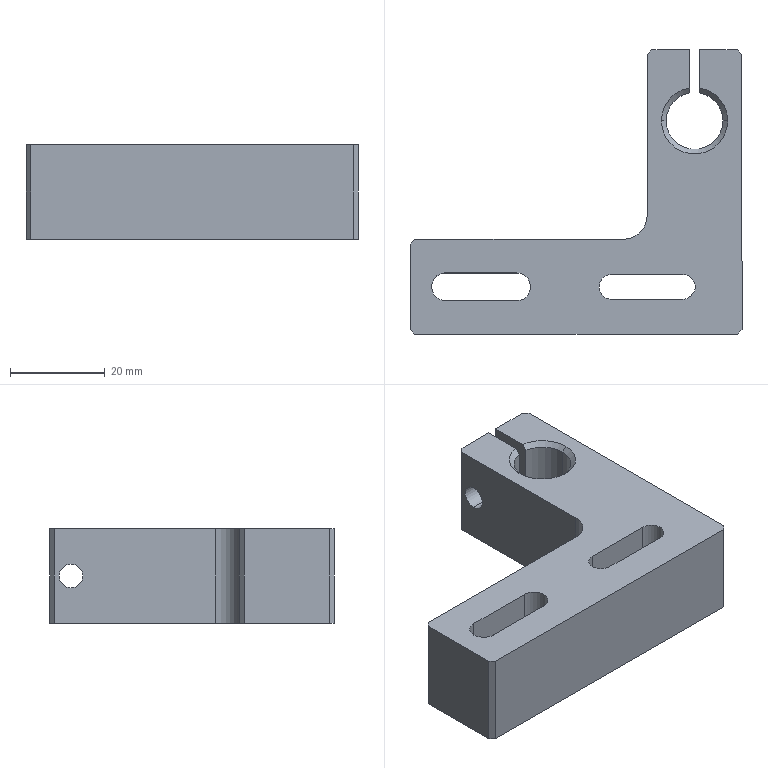Part | SolidWorks | features Chamfer 2, HoleWzd 2, Extrusion 1, Fillet 1 | 1 solid | 40 faces | box 70 x 60 x 20 mm | volume 36605 mm3 | plane 20 | cylinder 14 | cone 6 | commonest cylinder face diameters 5.256 x3 5.858 x3 12 x3 5 x2 6.6 x2 10 x1
STEP:
#1=CARTESIAN_POINT('',(13.05,30.296,13.3));
#2=VERTEX_POINT('',#1);
#3=CARTESIAN_POINT('',(13.05,30.296,6.7));
#4=VERTEX_POINT('',#3);
#5=CARTESIAN_POINT('',(13.05,30.296,10.));
#6=DIRECTION('',(1.,0.,0.));
#7=DIRECTION('',(0.,0.,-1.));
#8=AXIS2_PLACEMENT_3D('',#5,#6,#7);
#9=CIRCLE('',#8,3.3);
#10=EDGE_CURVE('',#2,#4,#9,.T.);
#11=ORIENTED_EDGE('',*,*,#10,.F.);
#12=CARTESIAN_POINT('',(22.05,30.296,13.3));
#13=VERTEX_POINT('',#12);
#14=CARTESIAN_POINT('',(22.05,30.296,13.3));
#15=DIRECTION('',(1.,0.,0.));
#16=VECTOR('',#15,1000.);
#17=LINE('',#14,#16);
#18=EDGE_CURVE('',#2,#13,#17,.T.);
#19=ORIENTED_EDGE('',*,*,#18,.T.);
#20=CARTESIAN_POINT('',(22.05,30.296,6.7));
#21=VERTEX_POINT('',#20);
#22=CARTESIAN_POINT('',(22.05,30.296,10.));
#23=DIRECTION('',(1.,0.,0.));
#24=DIRECTION('',(0.,0.,-1.));
#25=AXIS2_PLACEMENT_3D('',#22,#23,#24);
#26=CIRCLE('',#25,3.3);
#27=EDGE_CURVE('',#13,#21,#26,.T.);
#28=ORIENTED_EDGE('',*,*,#27,.T.);
#29=CARTESIAN_POINT('',(22.05,30.296,6.7));
#30=DIRECTION('',(1.,0.,0.));
#31=VECTOR('',#30,1000.);
#32=LINE('',#29,#31);
#33=EDGE_CURVE('',#4,#21,#32,.T.);
#34=ORIENTED_EDGE('',*,*,#33,.F.);
#35=EDGE_LOOP('',(#11,#19,#28,#34));
#36=FACE_OUTER_BOUND('',#35,.T.);
#37=CARTESIAN_POINT('',(22.05,30.296,10.));
#38=DIRECTION('',(1.,0.,0.));
#39=DIRECTION('',(0.,0.,-1.));
#40=AXIS2_PLACEMENT_3D('',#37,#38,#39);
#41=CYLINDRICAL_SURFACE('',#40,3.3);
#42=ADVANCED_FACE('',(#36),#41,.F.);
#43=CARTESIAN_POINT('',(11.05,30.296,7.5));
#44=VERTEX_POINT('',#43);
#45=CARTESIAN_POINT('',(11.05,30.296,12.5));
#46=VERTEX_POINT('',#45);
#47=CARTESIAN_POINT('',(11.05,30.296,10.));
#48=DIRECTION('',(-1.,0.,0.));
#49=DIRECTION('',(0.,0.,1.));
#50=AXIS2_PLACEMENT_3D('',#47,#48,#49);
#51=CIRCLE('',#50,2.5);
#52=EDGE_CURVE('',#44,#46,#51,.T.);
#53=ORIENTED_EDGE('',*,*,#52,.F.);
#54=CARTESIAN_POINT('',(2.05,30.296,7.5));
#55=VERTEX_POINT('',#54);
#56=CARTESIAN_POINT('',(2.05,30.296,7.5));
#57=DIRECTION('',(-1.,0.,0.));
#58=VECTOR('',#57,1000.);
#59=LINE('',#56,#58);
#60=EDGE_CURVE('',#44,#55,#59,.T.);
#61=ORIENTED_EDGE('',*,*,#60,.T.);
#62=CARTESIAN_POINT('',(2.05,30.296,12.5));
#63=VERTEX_POINT('',#62);
#64=CARTESIAN_POINT('',(2.05,30.296,10.));
#65=DIRECTION('',(-1.,0.,0.));
#66=DIRECTION('',(0.,0.,1.));
#67=AXIS2_PLACEMENT_3D('',#64,#65,#66);
#68=CIRCLE('',#67,2.5);
#69=EDGE_CURVE('',#55,#63,#68,.T.);
#70=ORIENTED_EDGE('',*,*,#69,.T.);
#71=CARTESIAN_POINT('',(2.05,30.296,12.5));
#72=DIRECTION('',(-1.,0.,0.));
#73=VECTOR('',#72,1000.);
#74=LINE('',#71,#73);
#75=EDGE_CURVE('',#46,#63,#74,.T.);
#76=ORIENTED_EDGE('',*,*,#75,.F.);
#77=EDGE_LOOP('',(#53,#61,#70,#76));
#78=FACE_OUTER_BOUND('',#77,.T.);
#79=CARTESIAN_POINT('',(2.05,30.296,10.));
#80=DIRECTION('',(-1.,0.,0.));
#81=DIRECTION('',(0.,0.,1.));
#82=AXIS2_PLACEMENT_3D('',#79,#80,#81);
#83=CYLINDRICAL_SURFACE('',#82,2.5);
#84=ADVANCED_FACE('',(#78),#83,.F.);
#85=CARTESIAN_POINT('',(6.05,19.796,19.));
#86=VERTEX_POINT('',#85);
#87=CARTESIAN_POINT('',(18.05,19.796,19.));
#88=VERTEX_POINT('',#87);
#89=CARTESIAN_POINT('',(12.05,19.796,19.));
#90=DIRECTION('',(0.,0.,1.));
#91=DIRECTION('',(1.,0.,0.));
#92=AXIS2_PLACEMENT_3D('',#89,#90,#91);
#93=CIRCLE('',#92,6.);
#94=EDGE_CURVE('',#86,#88,#93,.T.);
#95=ORIENTED_EDGE('',*,*,#94,.F.);
#96=CARTESIAN_POINT('',(5.05,19.796,20.));
#97=VERTEX_POINT('',#96);
#98=CARTESIAN_POINT('',(5.05,19.796,20.));
#99=DIRECTION('',(-0.7071,0.,0.7071));
#100=VECTOR('',#99,1000.);
#101=LINE('',#98,#100);
#102=EDGE_CURVE('',#86,#97,#101,.T.);
#103=ORIENTED_EDGE('',*,*,#102,.T.);
#104=CARTESIAN_POINT('',(19.05,19.796,20.));
#105=VERTEX_POINT('',#104);
#106=CARTESIAN_POINT('',(12.05,19.796,20.));
#107=DIRECTION('',(0.,0.,-1.));
#108=DIRECTION('',(1.,0.,0.));
#109=AXIS2_PLACEMENT_3D('',#106,#107,#108);
#110=CIRCLE('',#109,7.);
#111=EDGE_CURVE('',#105,#97,#110,.T.);
#112=ORIENTED_EDGE('',*,*,#111,.F.);
#113=CARTESIAN_POINT('',(19.05,19.796,20.));
#114=DIRECTION('',(0.7071,0.,0.7071));
#115=VECTOR('',#114,1000.);
#116=LINE('',#113,#115);
#117=EDGE_CURVE('',#88,#105,#116,.T.);
#118=ORIENTED_EDGE('',*,*,#117,.F.);
#119=EDGE_LOOP('',(#95,#103,#112,#118));
#120=FACE_OUTER_BOUND('',#119,.T.);
#121=CARTESIAN_POINT('',(12.05,19.796,20.));
#122=DIRECTION('',(0.,0.,1.));
#123=DIRECTION('',(1.,0.,0.));
#124=AXIS2_PLACEMENT_3D('',#121,#122,#123);
#125=CONICAL_SURFACE('',#124,7.,0.7854);
#126=ADVANCED_FACE('',(#120),#125,.F.);
#127=CARTESIAN_POINT('',(13.05,25.712,19.));
#128=VERTEX_POINT('',#127);
#129=CARTESIAN_POINT('',(12.05,19.796,19.));
#130=DIRECTION('',(0.,0.,1.));
#131=DIRECTION('',(1.,0.,0.));
#132=AXIS2_PLACEMENT_3D('',#129,#130,#131);
#133=CIRCLE('',#132,6.);
#134=EDGE_CURVE('',#88,#128,#133,.T.);
#135=ORIENTED_EDGE('',*,*,#134,.F.);
#136=ORIENTED_EDGE('',*,*,#117,.T.);
#137=CARTESIAN_POINT('',(13.05,26.724,20.));
#138=VERTEX_POINT('',#137);
#139=CARTESIAN_POINT('',(12.05,19.796,20.));
#140=DIRECTION('',(0.,0.,-1.));
#141=DIRECTION('',(1.,0.,0.));
#142=AXIS2_PLACEMENT_3D('',#139,#140,#141);
#143=CIRCLE('',#142,7.);
#144=EDGE_CURVE('',#138,#105,#143,.T.);
#145=ORIENTED_EDGE('',*,*,#144,.F.);
#146=CARTESIAN_POINT('',(13.05,25.712,19.));
#147=CARTESIAN_POINT('',(13.05,26.05,19.333));
#148=CARTESIAN_POINT('',(13.05,26.387,19.666));
#149=CARTESIAN_POINT('',(13.05,26.724,20.));
#150=B_SPLINE_CURVE_WITH_KNOTS('',3,(#146,#147,#148,#149),.UNSPECIFIED.,.F.,.F.,(4,4),(0.,0.001423),.UNSPECIFIED.);
#151=EDGE_CURVE('',#128,#138,#150,.T.);
#152=ORIENTED_EDGE('',*,*,#151,.F.);
#153=EDGE_LOOP('',(#135,#136,#145,#152));
#154=FACE_OUTER_BOUND('',#153,.T.);
#155=CARTESIAN_POINT('',(12.05,19.796,20.));
#156=DIRECTION('',(0.,0.,1.));
#157=DIRECTION('',(1.,0.,0.));
#158=AXIS2_PLACEMENT_3D('',#155,#156,#157);
#159=CONICAL_SURFACE('',#158,7.,0.7854);
#160=ADVANCED_FACE('',(#154),#159,.F.);
#161=CARTESIAN_POINT('',(18.05,19.796,1.));
#162=VERTEX_POINT('',#161);
#163=CARTESIAN_POINT('',(6.05,19.796,1.));
#164=VERTEX_POINT('',#163);
#165=CARTESIAN_POINT('',(12.05,19.796,1.));
#166=DIRECTION('',(0.,0.,-1.));
#167=DIRECTION('',(1.,0.,0.));
#168=AXIS2_PLACEMENT_3D('',#165,#166,#167);
#169=CIRCLE('',#168,6.);
#170=EDGE_CURVE('',#162,#164,#169,.T.);
#171=ORIENTED_EDGE('',*,*,#170,.F.);
#172=CARTESIAN_POINT('',(19.05,19.796,0.));
#173=VERTEX_POINT('',#172);
#174=CARTESIAN_POINT('',(18.05,19.796,1.));
#175=DIRECTION('',(0.7071,0.,-0.7071));
#176=VECTOR('',#175,1000.);
#177=LINE('',#174,#176);
#178=EDGE_CURVE('',#162,#173,#177,.T.);
#179=ORIENTED_EDGE('',*,*,#178,.T.);
#180=CARTESIAN_POINT('',(5.05,19.796,0.));
#181=VERTEX_POINT('',#180);
#182=CARTESIAN_POINT('',(12.05,19.796,0.));
#183=DIRECTION('',(0.,0.,1.));
#184=DIRECTION('',(1.,0.,0.));
#185=AXIS2_PLACEMENT_3D('',#182,#183,#184);
#186=CIRCLE('',#185,7.);
#187=EDGE_CURVE('',#181,#173,#186,.T.);
#188=ORIENTED_EDGE('',*,*,#187,.F.);
#189=CARTESIAN_POINT('',(6.05,19.796,1.));
#190=DIRECTION('',(-0.7071,0.,-0.7071));
#191=VECTOR('',#190,1000.);
#192=LINE('',#189,#191);
#193=EDGE_CURVE('',#164,#181,#192,.T.);
#194=ORIENTED_EDGE('',*,*,#193,.F.);
#195=EDGE_LOOP('',(#171,#179,#188,#194));
#196=FACE_OUTER_BOUND('',#195,.T.);
#197=CARTESIAN_POINT('',(12.05,19.796,1.));
#198=DIRECTION('',(0.,0.,-1.));
#199=DIRECTION('',(-1.,0.,0.));
#200=AXIS2_PLACEMENT_3D('',#197,#198,#199);
#201=CONICAL_SURFACE('',#200,6.,0.7854);
#202=ADVANCED_FACE('',(#196),#201,.F.);
#203=CARTESIAN_POINT('',(11.05,25.712,1.));
#204=VERTEX_POINT('',#203);
#205=CARTESIAN_POINT('',(12.05,19.796,1.));
#206=DIRECTION('',(0.,0.,-1.));
#207=DIRECTION('',(1.,0.,0.));
#208=AXIS2_PLACEMENT_3D('',#205,#206,#207);
#209=CIRCLE('',#208,6.);
#210=EDGE_CURVE('',#164,#204,#209,.T.);
#211=ORIENTED_EDGE('',*,*,#210,.F.);
#212=ORIENTED_EDGE('',*,*,#193,.T.);
#213=CARTESIAN_POINT('',(11.05,26.724,0.));
#214=VERTEX_POINT('',#213);
#215=CARTESIAN_POINT('',(12.05,19.796,0.));
#216=DIRECTION('',(0.,0.,1.));
#217=DIRECTION('',(1.,0.,0.));
#218=AXIS2_PLACEMENT_3D('',#215,#216,#217);
#219=CIRCLE('',#218,7.);
#220=EDGE_CURVE('',#214,#181,#219,.T.);
#221=ORIENTED_EDGE('',*,*,#220,.F.);
#222=CARTESIAN_POINT('',(11.05,25.712,1.));
#223=CARTESIAN_POINT('',(11.05,26.05,0.667));
#224=CARTESIAN_POINT('',(11.05,26.387,0.3336));
#225=CARTESIAN_POINT('',(11.05,26.724,0.));
#226=B_SPLINE_CURVE_WITH_KNOTS('',3,(#222,#223,#224,#225),.UNSPECIFIED.,.F.,.F.,(4,4),(0.,0.001423),.UNSPECIFIED.);
#227=EDGE_CURVE('',#204,#214,#226,.T.);
#228=ORIENTED_EDGE('',*,*,#227,.F.);
#229=EDGE_LOOP('',(#211,#212,#221,#228));
#230=FACE_OUTER_BOUND('',#229,.T.);
#231=CARTESIAN_POINT('',(12.05,19.796,1.));
#232=DIRECTION('',(0.,0.,-1.));
#233=DIRECTION('',(-1.,0.,0.));
#234=AXIS2_PLACEMENT_3D('',#231,#232,#233);
#235=CONICAL_SURFACE('',#234,6.,0.7854);
#236=ADVANCED_FACE('',(#230),#235,.F.);
#237=CARTESIAN_POINT('',(-5.45,-12.576,20.));
#238=VERTEX_POINT('',#237);
#239=CARTESIAN_POINT('',(-8.078,-15.204,20.));
#240=VERTEX_POINT('',#239);
#241=CARTESIAN_POINT('',(-5.45,-15.204,20.));
#242=DIRECTION('',(0.,0.,1.));
#243=DIRECTION('',(1.,0.,0.));
#244=AXIS2_PLACEMENT_3D('',#241,#242,#243);
#245=CIRCLE('',#244,2.628);
#246=EDGE_CURVE('',#238,#240,#245,.T.);
#247=ORIENTED_EDGE('',*,*,#246,.T.);
#248=CARTESIAN_POINT('',(-8.078,-15.204,0.));
#249=VERTEX_POINT('',#248);
#250=CARTESIAN_POINT('',(-8.078,-15.204,20.));
#251=DIRECTION('',(0.,0.,-1.));
#252=VECTOR('',#251,1000.);
#253=LINE('',#250,#252);
#254=EDGE_CURVE('',#240,#249,#253,.T.);
#255=ORIENTED_EDGE('',*,*,#254,.T.);
#256=CARTESIAN_POINT('',(-5.45,-12.576,0.));
#257=VERTEX_POINT('',#256);
#258=CARTESIAN_POINT('',(-5.45,-15.204,0.));
#259=DIRECTION('',(0.,0.,1.));
#260=DIRECTION('',(1.,0.,0.));
#261=AXIS2_PLACEMENT_3D('',#258,#259,#260);
#262=CIRCLE('',#261,2.628);
#263=EDGE_CURVE('',#257,#249,#262,.T.);
#264=ORIENTED_EDGE('',*,*,#263,.F.);
#265=CARTESIAN_POINT('',(-5.45,-12.576,20.));
#266=DIRECTION('',(0.,0.,-1.));
#267=VECTOR('',#266,1000.);
#268=LINE('',#265,#267);
#269=EDGE_CURVE('',#238,#257,#268,.T.);
#270=ORIENTED_EDGE('',*,*,#269,.F.);
#271=EDGE_LOOP('',(#247,#255,#264,#270));
#272=FACE_OUTER_BOUND('',#271,.T.);
#273=CARTESIAN_POINT('',(-5.45,-15.204,20.));
#274=DIRECTION('',(0.,0.,-1.));
#275=DIRECTION('',(-1.,0.,0.));
#276=AXIS2_PLACEMENT_3D('',#273,#274,#275);
#277=CYLINDRICAL_SURFACE('',#276,2.628);
#278=ADVANCED_FACE('',(#272),#277,.F.);
#279=CARTESIAN_POINT('',(-40.45,-12.275,20.));
#280=VERTEX_POINT('',#279);
#281=CARTESIAN_POINT('',(-43.379,-15.204,20.));
#282=VERTEX_POINT('',#281);
#283=CARTESIAN_POINT('',(-40.45,-15.204,20.));
#284=DIRECTION('',(0.,0.,1.));
#285=DIRECTION('',(1.,0.,0.));
#286=AXIS2_PLACEMENT_3D('',#283,#284,#285);
#287=CIRCLE('',#286,2.929);
#288=EDGE_CURVE('',#280,#282,#287,.T.);
#289=ORIENTED_EDGE('',*,*,#288,.T.);
#290=CARTESIAN_POINT('',(-43.379,-15.204,0.));
#291=VERTEX_POINT('',#290);
#292=CARTESIAN_POINT('',(-43.379,-15.204,20.));
#293=DIRECTION('',(0.,0.,-1.));
#294=VECTOR('',#293,1000.);
#295=LINE('',#292,#294);
#296=EDGE_CURVE('',#282,#291,#295,.T.);
#297=ORIENTED_EDGE('',*,*,#296,.T.);
#298=CARTESIAN_POINT('',(-40.45,-12.275,0.));
#299=VERTEX_POINT('',#298);
#300=CARTESIAN_POINT('',(-40.45,-15.204,0.));
#301=DIRECTION('',(0.,0.,1.));
#302=DIRECTION('',(1.,0.,0.));
#303=AXIS2_PLACEMENT_3D('',#300,#301,#302);
#304=CIRCLE('',#303,2.929);
#305=EDGE_CURVE('',#299,#291,#304,.T.);
#306=ORIENTED_EDGE('',*,*,#305,.F.);
#307=CARTESIAN_POINT('',(-40.45,-12.275,20.));
#308=DIRECTION('',(0.,0.,-1.));
#309=VECTOR('',#308,1000.);
#310=LINE('',#307,#309);
#311=EDGE_CURVE('',#280,#299,#310,.T.);
#312=ORIENTED_EDGE('',*,*,#311,.F.);
#313=EDGE_LOOP('',(#289,#297,#306,#312));
#314=FACE_OUTER_BOUND('',#313,.T.);
#315=CARTESIAN_POINT('',(-40.45,-15.204,20.));
#316=DIRECTION('',(0.,0.,-1.));
#317=DIRECTION('',(-1.,0.,0.));
#318=AXIS2_PLACEMENT_3D('',#315,#316,#317);
#319=CYLINDRICAL_SURFACE('',#318,2.929);
#320=ADVANCED_FACE('',(#314),#319,.F.);
#321=ORIENTED_EDGE('',*,*,#94,.T.);
#322=CARTESIAN_POINT('',(18.05,19.796,20.));
#323=DIRECTION('',(0.,0.,-1.));
#324=VECTOR('',#323,1000.);
#325=LINE('',#322,#324);
#326=EDGE_CURVE('',#88,#162,#325,.T.);
#327=ORIENTED_EDGE('',*,*,#326,.T.);
#328=ORIENTED_EDGE('',*,*,#170,.T.);
#329=CARTESIAN_POINT('',(6.05,19.796,20.));
#330=DIRECTION('',(0.,0.,-1.));
#331=VECTOR('',#330,1000.);
#332=LINE('',#329,#331);
#333=EDGE_CURVE('',#86,#164,#332,.T.);
#334=ORIENTED_EDGE('',*,*,#333,.F.);
#335=EDGE_LOOP('',(#321,#327,#328,#334));
#336=FACE_OUTER_BOUND('',#335,.T.);
#337=CARTESIAN_POINT('',(12.05,19.796,20.));
#338=DIRECTION('',(0.,0.,-1.));
#339=DIRECTION('',(-1.,0.,0.));
#340=AXIS2_PLACEMENT_3D('',#337,#338,#339);
#341=CYLINDRICAL_SURFACE('',#340,6.);
#342=ADVANCED_FACE('',(#336),#341,.F.);
#343=CARTESIAN_POINT('',(11.05,25.712,19.));
#344=VERTEX_POINT('',#343);
#345=CARTESIAN_POINT('',(12.05,19.796,19.));
#346=DIRECTION('',(0.,0.,1.));
#347=DIRECTION('',(1.,0.,0.));
#348=AXIS2_PLACEMENT_3D('',#345,#346,#347);
#349=CIRCLE('',#348,6.);
#350=EDGE_CURVE('',#344,#86,#349,.T.);
#351=ORIENTED_EDGE('',*,*,#350,.T.);
#352=ORIENTED_EDGE('',*,*,#333,.T.);
#353=ORIENTED_EDGE('',*,*,#210,.T.);
#354=CARTESIAN_POINT('',(11.05,25.712,20.));
#355=DIRECTION('',(0.,0.,-1.));
#356=VECTOR('',#355,1000.);
#357=LINE('',#354,#356);
#358=EDGE_CURVE('',#344,#204,#357,.T.);
#359=ORIENTED_EDGE('',*,*,#358,.F.);
#360=EDGE_LOOP('',(#351,#352,#353,#359));
#361=FACE_OUTER_BOUND('',#360,.T.);
#362=CARTESIAN_POINT('',(12.05,19.796,20.));
#363=DIRECTION('',(0.,0.,-1.));
#364=DIRECTION('',(-1.,0.,0.));
#365=AXIS2_PLACEMENT_3D('',#362,#363,#364);
#366=CYLINDRICAL_SURFACE('',#365,6.);
#367=ADVANCED_FACE('',(#361),#366,.F.);
#368=CARTESIAN_POINT('',(-47.95,-6.204,20.));
#369=VERTEX_POINT('',#368);
#370=CARTESIAN_POINT('',(-47.95,-24.204,20.));
#371=VERTEX_POINT('',#370);
#372=CARTESIAN_POINT('',(-47.95,-25.204,20.));
#373=DIRECTION('',(0.,-1.,0.));
#374=VECTOR('',#373,1000.);
#375=LINE('',#372,#374);
#376=EDGE_CURVE('',#369,#371,#375,.T.);
#377=ORIENTED_EDGE('',*,*,#376,.T.);
#378=CARTESIAN_POINT('',(-46.95,-25.204,20.));
#379=VERTEX_POINT('',#378);
#380=CARTESIAN_POINT('',(-39.95,-32.204,20.));
#381=DIRECTION('',(0.7071,-0.7071,0.));
#382=VECTOR('',#381,1000.);
#383=LINE('',#380,#382);
#384=EDGE_CURVE('',#371,#379,#383,.T.);
#385=ORIENTED_EDGE('',*,*,#384,.T.);
#386=CARTESIAN_POINT('',(21.05,-25.204,20.));
#387=VERTEX_POINT('',#386);
#388=CARTESIAN_POINT('',(22.05,-25.204,20.));
#389=DIRECTION('',(1.,0.,0.));
#390=VECTOR('',#389,1000.);
#391=LINE('',#388,#390);
#392=EDGE_CURVE('',#379,#387,#391,.T.);
#393=ORIENTED_EDGE('',*,*,#392,.T.);
#394=CARTESIAN_POINT('',(22.05,-24.204,20.));
#395=VERTEX_POINT('',#394);
#396=CARTESIAN_POINT('',(39.05,-7.204,20.));
#397=DIRECTION('',(0.7071,0.7071,0.));
#398=VECTOR('',#397,1000.);
#399=LINE('',#396,#398);
#400=EDGE_CURVE('',#387,#395,#399,.T.);
#401=ORIENTED_EDGE('',*,*,#400,.T.);
#402=CARTESIAN_POINT('',(22.05,33.796,20.));
#403=VERTEX_POINT('',#402);
#404=CARTESIAN_POINT('',(22.05,34.796,20.));
#405=DIRECTION('',(0.,1.,0.));
#406=VECTOR('',#405,1000.);
#407=LINE('',#404,#406);
#408=EDGE_CURVE('',#395,#403,#407,.T.);
#409=ORIENTED_EDGE('',*,*,#408,.T.);
#410=CARTESIAN_POINT('',(21.05,34.796,20.));
#411=VERTEX_POINT('',#410);
#412=CARTESIAN_POINT('',(24.05,31.796,20.));
#413=DIRECTION('',(-0.7071,0.7071,0.));
#414=VECTOR('',#413,1000.);
#415=LINE('',#412,#414);
#416=EDGE_CURVE('',#403,#411,#415,.T.);
#417=ORIENTED_EDGE('',*,*,#416,.T.);
#418=CARTESIAN_POINT('',(13.05,34.796,20.));
#419=VERTEX_POINT('',#418);
#420=CARTESIAN_POINT('',(13.05,34.796,20.));
#421=DIRECTION('',(-1.,0.,0.));
#422=VECTOR('',#421,1000.);
#423=LINE('',#420,#422);
#424=EDGE_CURVE('',#411,#419,#423,.T.);
#425=ORIENTED_EDGE('',*,*,#424,.T.);
#426=CARTESIAN_POINT('',(13.05,34.796,20.));
#427=DIRECTION('',(0.,-1.,0.));
#428=VECTOR('',#427,1000.);
#429=LINE('',#426,#428);
#430=EDGE_CURVE('',#419,#138,#429,.T.);
#431=ORIENTED_EDGE('',*,*,#430,.T.);
#432=ORIENTED_EDGE('',*,*,#144,.T.);
#433=ORIENTED_EDGE('',*,*,#111,.T.);
#434=CARTESIAN_POINT('',(11.05,26.724,20.));
#435=VERTEX_POINT('',#434);
#436=CARTESIAN_POINT('',(12.05,19.796,20.));
#437=DIRECTION('',(0.,0.,-1.));
#438=DIRECTION('',(1.,0.,0.));
#439=AXIS2_PLACEMENT_3D('',#436,#437,#438);
#440=CIRCLE('',#439,7.);
#441=EDGE_CURVE('',#97,#435,#440,.T.);
#442=ORIENTED_EDGE('',*,*,#441,.T.);
#443=CARTESIAN_POINT('',(11.05,34.796,20.));
#444=VERTEX_POINT('',#443);
#445=CARTESIAN_POINT('',(11.05,34.796,20.));
#446=DIRECTION('',(0.,1.,0.));
#447=VECTOR('',#446,1000.);
#448=LINE('',#445,#447);
#449=EDGE_CURVE('',#435,#444,#448,.T.);
#450=ORIENTED_EDGE('',*,*,#449,.T.);
#451=CARTESIAN_POINT('',(3.05,34.796,20.));
#452=VERTEX_POINT('',#451);
#453=CARTESIAN_POINT('',(2.05,34.796,20.));
#454=DIRECTION('',(-1.,0.,0.));
#455=VECTOR('',#454,1000.);
#456=LINE('',#453,#455);
#457=EDGE_CURVE('',#444,#452,#456,.T.);
#458=ORIENTED_EDGE('',*,*,#457,.T.);
#459=CARTESIAN_POINT('',(2.05,33.796,20.));
#460=VERTEX_POINT('',#459);
#461=CARTESIAN_POINT('',(0.04994,31.796,20.));
#462=DIRECTION('',(-0.7071,-0.7071,0.));
#463=VECTOR('',#462,1000.);
#464=LINE('',#461,#463);
#465=EDGE_CURVE('',#452,#460,#464,.T.);
#466=ORIENTED_EDGE('',*,*,#465,.T.);
#467=CARTESIAN_POINT('',(2.05,-0.2041,20.));
#468=VERTEX_POINT('',#467);
#469=CARTESIAN_POINT('',(2.05,-5.204,20.));
#470=DIRECTION('',(0.,-1.,0.));
#471=VECTOR('',#470,1000.);
#472=LINE('',#469,#471);
#473=EDGE_CURVE('',#460,#468,#472,.T.);
#474=ORIENTED_EDGE('',*,*,#473,.T.);
#475=CARTESIAN_POINT('',(-2.95,-5.204,20.));
#476=VERTEX_POINT('',#475);
#477=CARTESIAN_POINT('',(-2.95,-0.2041,20.));
#478=DIRECTION('',(0.,0.,-1.));
#479=DIRECTION('',(1.,0.,0.));
#480=AXIS2_PLACEMENT_3D('',#477,#478,#479);
#481=CIRCLE('',#480,5.);
#482=EDGE_CURVE('',#468,#476,#481,.T.);
#483=ORIENTED_EDGE('',*,*,#482,.T.);
#484=CARTESIAN_POINT('',(-46.95,-5.204,20.));
#485=VERTEX_POINT('',#484);
#486=CARTESIAN_POINT('',(-47.95,-5.204,20.));
#487=DIRECTION('',(-1.,0.,0.));
#488=VECTOR('',#487,1000.);
#489=LINE('',#486,#488);
#490=EDGE_CURVE('',#476,#485,#489,.T.);
#491=ORIENTED_EDGE('',*,*,#490,.T.);
#492=CARTESIAN_POINT('',(-4.95,36.796,20.));
#493=DIRECTION('',(-0.7071,-0.7071,0.));
#494=VECTOR('',#493,1000.);
#495=LINE('',#492,#494);
#496=EDGE_CURVE('',#485,#369,#495,.T.);
#497=ORIENTED_EDGE('',*,*,#496,.T.);
#498=EDGE_LOOP('',(#377,#385,#393,#401,#409,#417,#425,#431,#432,#433,#442,#450,#458,#466,#474,#483,#491,#497));
#499=FACE_OUTER_BOUND('',#498,.T.);
#500=CARTESIAN_POINT('',(-40.45,-18.133,20.));
#501=VERTEX_POINT('',#500);
#502=CARTESIAN_POINT('',(-25.45,-18.133,20.));
#503=VERTEX_POINT('',#502);
#504=CARTESIAN_POINT('',(-40.45,-18.133,20.));
#505=DIRECTION('',(1.,0.,0.));
#506=VECTOR('',#505,1000.);
#507=LINE('',#504,#506);
#508=EDGE_CURVE('',#501,#503,#507,.T.);
#509=ORIENTED_EDGE('',*,*,#508,.F.);
#510=CARTESIAN_POINT('',(-40.45,-15.204,20.));
#511=DIRECTION('',(0.,0.,1.));
#512=DIRECTION('',(1.,0.,0.));
#513=AXIS2_PLACEMENT_3D('',#510,#511,#512);
#514=CIRCLE('',#513,2.929);
#515=EDGE_CURVE('',#282,#501,#514,.T.);
#516=ORIENTED_EDGE('',*,*,#515,.F.);
#517=ORIENTED_EDGE('',*,*,#288,.F.);
#518=CARTESIAN_POINT('',(-25.45,-12.275,20.));
#519=VERTEX_POINT('',#518);
#520=CARTESIAN_POINT('',(-40.45,-12.275,20.));
#521=DIRECTION('',(-1.,0.,0.));
#522=VECTOR('',#521,1000.);
#523=LINE('',#520,#522);
#524=EDGE_CURVE('',#519,#280,#523,.T.);
#525=ORIENTED_EDGE('',*,*,#524,.F.);
#526=CARTESIAN_POINT('',(-25.45,-15.204,20.));
#527=DIRECTION('',(0.,0.,1.));
#528=DIRECTION('',(1.,0.,0.));
#529=AXIS2_PLACEMENT_3D('',#526,#527,#528);
#530=CIRCLE('',#529,2.929);
#531=EDGE_CURVE('',#503,#519,#530,.T.);
#532=ORIENTED_EDGE('',*,*,#531,.F.);
#533=EDGE_LOOP('',(#509,#516,#517,#525,#532));
#534=FACE_BOUND('',#533,.T.);
#535=CARTESIAN_POINT('',(-5.45,-17.832,20.));
#536=VERTEX_POINT('',#535);
#537=CARTESIAN_POINT('',(9.55,-17.832,20.));
#538=VERTEX_POINT('',#537);
#539=CARTESIAN_POINT('',(-5.45,-17.832,20.));
#540=DIRECTION('',(1.,0.,0.));
#541=VECTOR('',#540,1000.);
#542=LINE('',#539,#541);
#543=EDGE_CURVE('',#536,#538,#542,.T.);
#544=ORIENTED_EDGE('',*,*,#543,.F.);
#545=CARTESIAN_POINT('',(-5.45,-15.204,20.));
#546=DIRECTION('',(0.,0.,1.));
#547=DIRECTION('',(1.,0.,0.));
#548=AXIS2_PLACEMENT_3D('',#545,#546,#547);
#549=CIRCLE('',#548,2.628);
#550=EDGE_CURVE('',#240,#536,#549,.T.);
#551=ORIENTED_EDGE('',*,*,#550,.F.);
#552=ORIENTED_EDGE('',*,*,#246,.F.);
#553=CARTESIAN_POINT('',(9.55,-12.576,20.));
#554=VERTEX_POINT('',#553);
#555=CARTESIAN_POINT('',(-5.45,-12.576,20.));
#556=DIRECTION('',(-1.,0.,0.));
#557=VECTOR('',#556,1000.);
#558=LINE('',#555,#557);
#559=EDGE_CURVE('',#554,#238,#558,.T.);
#560=ORIENTED_EDGE('',*,*,#559,.F.);
#561=CARTESIAN_POINT('',(9.55,-15.204,20.));
#562=DIRECTION('',(0.,0.,1.));
#563=DIRECTION('',(1.,0.,0.));
#564=AXIS2_PLACEMENT_3D('',#561,#562,#563);
#565=CIRCLE('',#564,2.628);
#566=EDGE_CURVE('',#538,#554,#565,.T.);
#567=ORIENTED_EDGE('',*,*,#566,.F.);
#568=EDGE_LOOP('',(#544,#551,#552,#560,#567));
#569=FACE_BOUND('',#568,.T.);
#570=CARTESIAN_POINT('',(12.05,19.796,20.));
#571=DIRECTION('',(0.,0.,1.));
#572=DIRECTION('',(1.,0.,0.));
#573=AXIS2_PLACEMENT_3D('',#570,#571,#572);
#574=PLANE('',#573);
#575=ADVANCED_FACE('',(#499,#534,#569),#574,.T.);
#576=ORIENTED_EDGE('',*,*,#305,.T.);
#577=CARTESIAN_POINT('',(-40.45,-18.133,0.));
#578=VERTEX_POINT('',#577);
#579=CARTESIAN_POINT('',(-40.45,-15.204,0.));
#580=DIRECTION('',(0.,0.,1.));
#581=DIRECTION('',(1.,0.,0.));
#582=AXIS2_PLACEMENT_3D('',#579,#580,#581);
#583=CIRCLE('',#582,2.929);
#584=EDGE_CURVE('',#291,#578,#583,.T.);
#585=ORIENTED_EDGE('',*,*,#584,.T.);
#586=CARTESIAN_POINT('',(-25.45,-18.133,0.));
#587=VERTEX_POINT('',#586);
#588=CARTESIAN_POINT('',(-40.45,-18.133,0.));
#589=DIRECTION('',(1.,0.,0.));
#590=VECTOR('',#589,1000.);
#591=LINE('',#588,#590);
#592=EDGE_CURVE('',#578,#587,#591,.T.);
#593=ORIENTED_EDGE('',*,*,#592,.T.);
#594=CARTESIAN_POINT('',(-25.45,-12.275,0.));
#595=VERTEX_POINT('',#594);
#596=CARTESIAN_POINT('',(-25.45,-15.204,0.));
#597=DIRECTION('',(0.,0.,1.));
#598=DIRECTION('',(1.,0.,0.));
#599=AXIS2_PLACEMENT_3D('',#596,#597,#598);
#600=CIRCLE('',#599,2.929);
#601=EDGE_CURVE('',#587,#595,#600,.T.);
#602=ORIENTED_EDGE('',*,*,#601,.T.);
#603=CARTESIAN_POINT('',(-40.45,-12.275,0.));
#604=DIRECTION('',(-1.,0.,0.));
#605=VECTOR('',#604,1000.);
#606=LINE('',#603,#605);
#607=EDGE_CURVE('',#595,#299,#606,.T.);
#608=ORIENTED_EDGE('',*,*,#607,.T.);
#609=EDGE_LOOP('',(#576,#585,#593,#602,#608));
#610=FACE_BOUND('',#609,.T.);
#611=CARTESIAN_POINT('',(-46.95,-25.204,0.));
#612=VERTEX_POINT('',#611);
#613=CARTESIAN_POINT('',(21.05,-25.204,0.));
#614=VERTEX_POINT('',#613);
#615=CARTESIAN_POINT('',(22.05,-25.204,0.));
#616=DIRECTION('',(1.,0.,0.));
#617=VECTOR('',#616,1000.);
#618=LINE('',#615,#617);
#619=EDGE_CURVE('',#612,#614,#618,.T.);
#620=ORIENTED_EDGE('',*,*,#619,.F.);
#621=CARTESIAN_POINT('',(-47.95,-24.204,0.));
#622=VERTEX_POINT('',#621);
#623=CARTESIAN_POINT('',(-46.95,-25.204,0.));
#624=DIRECTION('',(-0.7071,0.7071,0.));
#625=VECTOR('',#624,1000.);
#626=LINE('',#623,#625);
#627=EDGE_CURVE('',#612,#622,#626,.T.);
#628=ORIENTED_EDGE('',*,*,#627,.T.);
#629=CARTESIAN_POINT('',(-47.95,-6.204,0.));
#630=VERTEX_POINT('',#629);
#631=CARTESIAN_POINT('',(-47.95,-25.204,0.));
#632=DIRECTION('',(0.,-1.,0.));
#633=VECTOR('',#632,1000.);
#634=LINE('',#631,#633);
#635=EDGE_CURVE('',#630,#622,#634,.T.);
#636=ORIENTED_EDGE('',*,*,#635,.F.);
#637=CARTESIAN_POINT('',(-46.95,-5.204,0.));
#638=VERTEX_POINT('',#637);
#639=CARTESIAN_POINT('',(-47.95,-6.204,0.));
#640=DIRECTION('',(0.7071,0.7071,0.));
#641=VECTOR('',#640,1000.);
#642=LINE('',#639,#641);
#643=EDGE_CURVE('',#630,#638,#642,.T.);
#644=ORIENTED_EDGE('',*,*,#643,.T.);
#645=CARTESIAN_POINT('',(-2.95,-5.204,0.));
#646=VERTEX_POINT('',#645);
#647=CARTESIAN_POINT('',(-47.95,-5.204,0.));
#648=DIRECTION('',(-1.,0.,0.));
#649=VECTOR('',#648,1000.);
#650=LINE('',#647,#649);
#651=EDGE_CURVE('',#646,#638,#650,.T.);
#652=ORIENTED_EDGE('',*,*,#651,.F.);
#653=CARTESIAN_POINT('',(2.05,-0.2041,0.));
#654=VERTEX_POINT('',#653);
#655=CARTESIAN_POINT('',(-2.95,-0.2041,0.));
#656=DIRECTION('',(0.,0.,1.));
#657=DIRECTION('',(1.,0.,0.));
#658=AXIS2_PLACEMENT_3D('',#655,#656,#657);
#659=CIRCLE('',#658,5.);
#660=EDGE_CURVE('',#646,#654,#659,.T.);
#661=ORIENTED_EDGE('',*,*,#660,.T.);
#662=CARTESIAN_POINT('',(2.05,33.796,0.));
#663=VERTEX_POINT('',#662);
#664=CARTESIAN_POINT('',(2.05,-5.204,0.));
#665=DIRECTION('',(0.,-1.,0.));
#666=VECTOR('',#665,1000.);
#667=LINE('',#664,#666);
#668=EDGE_CURVE('',#663,#654,#667,.T.);
#669=ORIENTED_EDGE('',*,*,#668,.F.);
#670=CARTESIAN_POINT('',(3.05,34.796,0.));
#671=VERTEX_POINT('',#670);
#672=CARTESIAN_POINT('',(2.05,33.796,0.));
#673=DIRECTION('',(0.7071,0.7071,0.));
#674=VECTOR('',#673,1000.);
#675=LINE('',#672,#674);
#676=EDGE_CURVE('',#663,#671,#675,.T.);
#677=ORIENTED_EDGE('',*,*,#676,.T.);
#678=CARTESIAN_POINT('',(11.05,34.796,0.));
#679=VERTEX_POINT('',#678);
#680=CARTESIAN_POINT('',(2.05,34.796,0.));
#681=DIRECTION('',(-1.,0.,0.));
#682=VECTOR('',#681,1000.);
#683=LINE('',#680,#682);
#684=EDGE_CURVE('',#679,#671,#683,.T.);
#685=ORIENTED_EDGE('',*,*,#684,.F.);
#686=CARTESIAN_POINT('',(11.05,34.796,0.));
#687=DIRECTION('',(0.,1.,0.));
#688=VECTOR('',#687,1000.);
#689=LINE('',#686,#688);
#690=EDGE_CURVE('',#214,#679,#689,.T.);
#691=ORIENTED_EDGE('',*,*,#690,.F.);
#692=ORIENTED_EDGE('',*,*,#220,.T.);
#693=ORIENTED_EDGE('',*,*,#187,.T.);
#694=CARTESIAN_POINT('',(13.05,26.724,0.));
#695=VERTEX_POINT('',#694);
#696=CARTESIAN_POINT('',(12.05,19.796,0.));
#697=DIRECTION('',(0.,0.,1.));
#698=DIRECTION('',(1.,0.,0.));
#699=AXIS2_PLACEMENT_3D('',#696,#697,#698);
#700=CIRCLE('',#699,7.);
#701=EDGE_CURVE('',#173,#695,#700,.T.);
#702=ORIENTED_EDGE('',*,*,#701,.T.);
#703=CARTESIAN_POINT('',(13.05,34.796,0.));
#704=VERTEX_POINT('',#703);
#705=CARTESIAN_POINT('',(13.05,34.796,0.));
#706=DIRECTION('',(0.,-1.,0.));
#707=VECTOR('',#706,1000.);
#708=LINE('',#705,#707);
#709=EDGE_CURVE('',#704,#695,#708,.T.);
#710=ORIENTED_EDGE('',*,*,#709,.F.);
#711=CARTESIAN_POINT('',(21.05,34.796,0.));
#712=VERTEX_POINT('',#711);
#713=CARTESIAN_POINT('',(13.05,34.796,0.));
#714=DIRECTION('',(-1.,0.,0.));
#715=VECTOR('',#714,1000.);
#716=LINE('',#713,#715);
#717=EDGE_CURVE('',#712,#704,#716,.T.);
#718=ORIENTED_EDGE('',*,*,#717,.F.);
#719=CARTESIAN_POINT('',(22.05,33.796,0.));
#720=VERTEX_POINT('',#719);
#721=CARTESIAN_POINT('',(21.05,34.796,0.));
#722=DIRECTION('',(0.7071,-0.7071,0.));
#723=VECTOR('',#722,1000.);
#724=LINE('',#721,#723);
#725=EDGE_CURVE('',#712,#720,#724,.T.);
#726=ORIENTED_EDGE('',*,*,#725,.T.);
#727=CARTESIAN_POINT('',(22.05,-24.204,0.));
#728=VERTEX_POINT('',#727);
#729=CARTESIAN_POINT('',(22.05,34.796,0.));
#730=DIRECTION('',(0.,1.,0.));
#731=VECTOR('',#730,1000.);
#732=LINE('',#729,#731);
#733=EDGE_CURVE('',#728,#720,#732,.T.);
#734=ORIENTED_EDGE('',*,*,#733,.F.);
#735=CARTESIAN_POINT('',(22.05,-24.204,0.));
#736=DIRECTION('',(-0.7071,-0.7071,0.));
#737=VECTOR('',#736,1000.);
#738=LINE('',#735,#737);
#739=EDGE_CURVE('',#728,#614,#738,.T.);
#740=ORIENTED_EDGE('',*,*,#739,.T.);
#741=EDGE_LOOP('',(#620,#628,#636,#644,#652,#661,#669,#677,#685,#691,#692,#693,#702,#710,#718,#726,#734,#740));
#742=FACE_OUTER_BOUND('',#741,.T.);
#743=ORIENTED_EDGE('',*,*,#263,.T.);
#744=CARTESIAN_POINT('',(-5.45,-17.832,0.));
#745=VERTEX_POINT('',#744);
#746=CARTESIAN_POINT('',(-5.45,-15.204,0.));
#747=DIRECTION('',(0.,0.,1.));
#748=DIRECTION('',(1.,0.,0.));
#749=AXIS2_PLACEMENT_3D('',#746,#747,#748);
#750=CIRCLE('',#749,2.628);
#751=EDGE_CURVE('',#249,#745,#750,.T.);
#752=ORIENTED_EDGE('',*,*,#751,.T.);
#753=CARTESIAN_POINT('',(9.55,-17.832,0.));
#754=VERTEX_POINT('',#753);
#755=CARTESIAN_POINT('',(-5.45,-17.832,0.));
#756=DIRECTION('',(1.,0.,0.));
#757=VECTOR('',#756,1000.);
#758=LINE('',#755,#757);
#759=EDGE_CURVE('',#745,#754,#758,.T.);
#760=ORIENTED_EDGE('',*,*,#759,.T.);
#761=CARTESIAN_POINT('',(9.55,-12.576,0.));
#762=VERTEX_POINT('',#761);
#763=CARTESIAN_POINT('',(9.55,-15.204,0.));
#764=DIRECTION('',(0.,0.,1.));
#765=DIRECTION('',(1.,0.,0.));
#766=AXIS2_PLACEMENT_3D('',#763,#764,#765);
#767=CIRCLE('',#766,2.628);
#768=EDGE_CURVE('',#754,#762,#767,.T.);
#769=ORIENTED_EDGE('',*,*,#768,.T.);
#770=CARTESIAN_POINT('',(-5.45,-12.576,0.));
#771=DIRECTION('',(-1.,0.,0.));
#772=VECTOR('',#771,1000.);
#773=LINE('',#770,#772);
#774=EDGE_CURVE('',#762,#257,#773,.T.);
#775=ORIENTED_EDGE('',*,*,#774,.T.);
#776=EDGE_LOOP('',(#743,#752,#760,#769,#775));
#777=FACE_BOUND('',#776,.T.);
#778=CARTESIAN_POINT('',(12.05,19.796,0.));
#779=DIRECTION('',(0.,0.,1.));
#780=DIRECTION('',(1.,0.,0.));
#781=AXIS2_PLACEMENT_3D('',#778,#779,#780);
#782=PLANE('',#781);
#783=ADVANCED_FACE('',(#610,#742,#777),#782,.F.);
#784=ORIENTED_EDGE('',*,*,#424,.F.);
#785=CARTESIAN_POINT('',(21.05,34.796,20.));
#786=DIRECTION('',(0.,0.,-1.));
#787=VECTOR('',#786,1000.);
#788=LINE('',#785,#787);
#789=EDGE_CURVE('',#411,#712,#788,.T.);
#790=ORIENTED_EDGE('',*,*,#789,.T.);
#791=ORIENTED_EDGE('',*,*,#717,.T.);
#792=CARTESIAN_POINT('',(13.05,34.796,20.));
#793=DIRECTION('',(0.,0.,-1.));
#794=VECTOR('',#793,1000.);
#795=LINE('',#792,#794);
#796=EDGE_CURVE('',#419,#704,#795,.T.);
#797=ORIENTED_EDGE('',*,*,#796,.F.);
#798=EDGE_LOOP('',(#784,#790,#791,#797));
#799=FACE_OUTER_BOUND('',#798,.T.);
#800=CARTESIAN_POINT('',(13.05,34.796,20.));
#801=DIRECTION('',(0.,-1.,0.));
#802=DIRECTION('',(0.,0.,-1.));
#803=AXIS2_PLACEMENT_3D('',#800,#801,#802);
#804=PLANE('',#803);
#805=ADVANCED_FACE('',(#799),#804,.F.);
#806=CARTESIAN_POINT('',(13.05,30.296,10.));
#807=DIRECTION('',(1.,0.,0.));
#808=DIRECTION('',(0.,0.,-1.));
#809=AXIS2_PLACEMENT_3D('',#806,#807,#808);
#810=CIRCLE('',#809,3.3);
#811=EDGE_CURVE('',#4,#2,#810,.T.);
#812=ORIENTED_EDGE('',*,*,#811,.T.);
#813=ORIENTED_EDGE('',*,*,#10,.T.);
#814=EDGE_LOOP('',(#812,#813));
#815=FACE_BOUND('',#814,.T.);
#816=ORIENTED_EDGE('',*,*,#709,.T.);
#817=CARTESIAN_POINT('',(13.05,25.712,1.));
#818=VERTEX_POINT('',#817);
#819=CARTESIAN_POINT('',(13.05,26.724,0.));
#820=CARTESIAN_POINT('',(13.05,26.387,0.3336));
#821=CARTESIAN_POINT('',(13.05,26.05,0.667));
#822=CARTESIAN_POINT('',(13.05,25.712,1.));
#823=B_SPLINE_CURVE_WITH_KNOTS('',3,(#819,#820,#821,#822),.UNSPECIFIED.,.F.,.F.,(4,4),(0.,0.001423),.UNSPECIFIED.);
#824=EDGE_CURVE('',#695,#818,#823,.T.);
#825=ORIENTED_EDGE('',*,*,#824,.T.);
#826=CARTESIAN_POINT('',(13.05,25.712,20.));
#827=DIRECTION('',(0.,0.,-1.));
#828=VECTOR('',#827,1000.);
#829=LINE('',#826,#828);
#830=EDGE_CURVE('',#128,#818,#829,.T.);
#831=ORIENTED_EDGE('',*,*,#830,.F.);
#832=ORIENTED_EDGE('',*,*,#151,.T.);
#833=ORIENTED_EDGE('',*,*,#430,.F.);
#834=ORIENTED_EDGE('',*,*,#796,.T.);
#835=EDGE_LOOP('',(#816,#825,#831,#832,#833,#834));
#836=FACE_OUTER_BOUND('',#835,.T.);
#837=CARTESIAN_POINT('',(13.05,34.796,20.));
#838=DIRECTION('',(1.,0.,0.));
#839=DIRECTION('',(0.,0.,-1.));
#840=AXIS2_PLACEMENT_3D('',#837,#838,#839);
#841=PLANE('',#840);
#842=ADVANCED_FACE('',(#815,#836),#841,.F.);
#843=ORIENTED_EDGE('',*,*,#326,.F.);
#844=ORIENTED_EDGE('',*,*,#134,.T.);
#845=ORIENTED_EDGE('',*,*,#830,.T.);
#846=CARTESIAN_POINT('',(12.05,19.796,1.));
#847=DIRECTION('',(0.,0.,-1.));
#848=DIRECTION('',(1.,0.,0.));
#849=AXIS2_PLACEMENT_3D('',#846,#847,#848);
#850=CIRCLE('',#849,6.);
#851=EDGE_CURVE('',#818,#162,#850,.T.);
#852=ORIENTED_EDGE('',*,*,#851,.T.);
#853=EDGE_LOOP('',(#843,#844,#845,#852));
#854=FACE_OUTER_BOUND('',#853,.T.);
#855=CARTESIAN_POINT('',(12.05,19.796,20.));
#856=DIRECTION('',(0.,0.,-1.));
#857=DIRECTION('',(-1.,0.,0.));
#858=AXIS2_PLACEMENT_3D('',#855,#856,#857);
#859=CYLINDRICAL_SURFACE('',#858,6.);
#860=ADVANCED_FACE('',(#854),#859,.F.);
#861=CARTESIAN_POINT('',(11.05,30.296,10.));
#862=DIRECTION('',(-1.,0.,0.));
#863=DIRECTION('',(0.,0.,1.));
#864=AXIS2_PLACEMENT_3D('',#861,#862,#863);
#865=CIRCLE('',#864,2.5);
#866=EDGE_CURVE('',#46,#44,#865,.T.);
#867=ORIENTED_EDGE('',*,*,#866,.T.);
#868=ORIENTED_EDGE('',*,*,#52,.T.);
#869=EDGE_LOOP('',(#867,#868));
#870=FACE_BOUND('',#869,.T.);
#871=ORIENTED_EDGE('',*,*,#358,.T.);
#872=ORIENTED_EDGE('',*,*,#227,.T.);
#873=ORIENTED_EDGE('',*,*,#690,.T.);
#874=CARTESIAN_POINT('',(11.05,34.796,20.));
#875=DIRECTION('',(0.,0.,-1.));
#876=VECTOR('',#875,1000.);
#877=LINE('',#874,#876);
#878=EDGE_CURVE('',#444,#679,#877,.T.);
#879=ORIENTED_EDGE('',*,*,#878,.F.);
#880=ORIENTED_EDGE('',*,*,#449,.F.);
#881=CARTESIAN_POINT('',(11.05,26.724,20.));
#882=CARTESIAN_POINT('',(11.05,26.387,19.666));
#883=CARTESIAN_POINT('',(11.05,26.05,19.333));
#884=CARTESIAN_POINT('',(11.05,25.712,19.));
#885=B_SPLINE_CURVE_WITH_KNOTS('',3,(#881,#882,#883,#884),.UNSPECIFIED.,.F.,.F.,(4,4),(0.,0.001423),.UNSPECIFIED.);
#886=EDGE_CURVE('',#435,#344,#885,.T.);
#887=ORIENTED_EDGE('',*,*,#886,.T.);
#888=EDGE_LOOP('',(#871,#872,#873,#879,#880,#887));
#889=FACE_OUTER_BOUND('',#888,.T.);
#890=CARTESIAN_POINT('',(11.05,34.796,20.));
#891=DIRECTION('',(-1.,0.,0.));
#892=DIRECTION('',(0.,0.,1.));
#893=AXIS2_PLACEMENT_3D('',#890,#891,#892);
#894=PLANE('',#893);
#895=ADVANCED_FACE('',(#870,#889),#894,.F.);
#896=ORIENTED_EDGE('',*,*,#684,.T.);
#897=CARTESIAN_POINT('',(3.05,34.796,20.));
#898=DIRECTION('',(0.,0.,1.));
#899=VECTOR('',#898,1000.);
#900=LINE('',#897,#899);
#901=EDGE_CURVE('',#671,#452,#900,.T.);
#902=ORIENTED_EDGE('',*,*,#901,.T.);
#903=ORIENTED_EDGE('',*,*,#457,.F.);
#904=ORIENTED_EDGE('',*,*,#878,.T.);
#905=EDGE_LOOP('',(#896,#902,#903,#904));
#906=FACE_OUTER_BOUND('',#905,.T.);
#907=CARTESIAN_POINT('',(2.05,34.796,20.));
#908=DIRECTION('',(0.,-1.,0.));
#909=DIRECTION('',(0.,0.,-1.));
#910=AXIS2_PLACEMENT_3D('',#907,#908,#909);
#911=PLANE('',#910);
#912=ADVANCED_FACE('',(#906),#911,.F.);
#913=CARTESIAN_POINT('',(2.05,30.296,10.));
#914=DIRECTION('',(-1.,0.,0.));
#915=DIRECTION('',(0.,0.,1.));
#916=AXIS2_PLACEMENT_3D('',#913,#914,#915);
#917=CIRCLE('',#916,2.5);
#918=EDGE_CURVE('',#63,#55,#917,.T.);
#919=ORIENTED_EDGE('',*,*,#918,.F.);
#920=ORIENTED_EDGE('',*,*,#69,.F.);
#921=EDGE_LOOP('',(#919,#920));
#922=FACE_BOUND('',#921,.T.);
#923=ORIENTED_EDGE('',*,*,#668,.T.);
#924=CARTESIAN_POINT('',(2.05,-0.2041,20.));
#925=DIRECTION('',(0.,0.,1.));
#926=VECTOR('',#925,1000.);
#927=LINE('',#924,#926);
#928=EDGE_CURVE('',#654,#468,#927,.T.);
#929=ORIENTED_EDGE('',*,*,#928,.T.);
#930=ORIENTED_EDGE('',*,*,#473,.F.);
#931=CARTESIAN_POINT('',(2.05,33.796,20.));
#932=DIRECTION('',(0.,0.,-1.));
#933=VECTOR('',#932,1000.);
#934=LINE('',#931,#933);
#935=EDGE_CURVE('',#460,#663,#934,.T.);
#936=ORIENTED_EDGE('',*,*,#935,.T.);
#937=EDGE_LOOP('',(#923,#929,#930,#936));
#938=FACE_OUTER_BOUND('',#937,.T.);
#939=CARTESIAN_POINT('',(2.05,-5.204,20.));
#940=DIRECTION('',(1.,0.,0.));
#941=DIRECTION('',(0.,1.,0.));
#942=AXIS2_PLACEMENT_3D('',#939,#940,#941);
#943=PLANE('',#942);
#944=ADVANCED_FACE('',(#922,#938),#943,.F.);
#945=ORIENTED_EDGE('',*,*,#490,.F.);
#946=CARTESIAN_POINT('',(-2.95,-5.204,0.));
#947=DIRECTION('',(0.,0.,-1.));
#948=VECTOR('',#947,1000.);
#949=LINE('',#946,#948);
#950=EDGE_CURVE('',#476,#646,#949,.T.);
#951=ORIENTED_EDGE('',*,*,#950,.T.);
#952=ORIENTED_EDGE('',*,*,#651,.T.);
#953=CARTESIAN_POINT('',(-46.95,-5.204,20.));
#954=DIRECTION('',(0.,0.,1.));
#955=VECTOR('',#954,1000.);
#956=LINE('',#953,#955);
#957=EDGE_CURVE('',#638,#485,#956,.T.);
#958=ORIENTED_EDGE('',*,*,#957,.T.);
#959=EDGE_LOOP('',(#945,#951,#952,#958));
#960=FACE_OUTER_BOUND('',#959,.T.);
#961=CARTESIAN_POINT('',(-47.95,-5.204,20.));
#962=DIRECTION('',(0.,-1.,0.));
#963=DIRECTION('',(0.,0.,-1.));
#964=AXIS2_PLACEMENT_3D('',#961,#962,#963);
#965=PLANE('',#964);
#966=ADVANCED_FACE('',(#960),#965,.F.);
#967=ORIENTED_EDGE('',*,*,#635,.T.);
#968=CARTESIAN_POINT('',(-47.95,-24.204,20.));
#969=DIRECTION('',(0.,0.,1.));
#970=VECTOR('',#969,1000.);
#971=LINE('',#968,#970);
#972=EDGE_CURVE('',#622,#371,#971,.T.);
#973=ORIENTED_EDGE('',*,*,#972,.T.);
#974=ORIENTED_EDGE('',*,*,#376,.F.);
#975=CARTESIAN_POINT('',(-47.95,-6.204,20.));
#976=DIRECTION('',(0.,0.,-1.));
#977=VECTOR('',#976,1000.);
#978=LINE('',#975,#977);
#979=EDGE_CURVE('',#369,#630,#978,.T.);
#980=ORIENTED_EDGE('',*,*,#979,.T.);
#981=EDGE_LOOP('',(#967,#973,#974,#980));
#982=FACE_OUTER_BOUND('',#981,.T.);
#983=CARTESIAN_POINT('',(-47.95,-25.204,20.));
#984=DIRECTION('',(1.,0.,0.));
#985=DIRECTION('',(0.,1.,0.));
#986=AXIS2_PLACEMENT_3D('',#983,#984,#985);
#987=PLANE('',#986);
#988=ADVANCED_FACE('',(#982),#987,.F.);
#989=ORIENTED_EDGE('',*,*,#392,.F.);
#990=CARTESIAN_POINT('',(-46.95,-25.204,20.));
#991=DIRECTION('',(0.,0.,-1.));
#992=VECTOR('',#991,1000.);
#993=LINE('',#990,#992);
#994=EDGE_CURVE('',#379,#612,#993,.T.);
#995=ORIENTED_EDGE('',*,*,#994,.T.);
#996=ORIENTED_EDGE('',*,*,#619,.T.);
#997=CARTESIAN_POINT('',(21.05,-25.204,20.));
#998=DIRECTION('',(0.,0.,1.));
#999=VECTOR('',#998,1000.);
#1000=LINE('',#997,#999);
#1001=EDGE_CURVE('',#614,#387,#1000,.T.);
#1002=ORIENTED_EDGE('',*,*,#1001,.T.);
#1003=EDGE_LOOP('',(#989,#995,#996,#1002));
#1004=FACE_OUTER_BOUND('',#1003,.T.);
#1005=CARTESIAN_POINT('',(22.05,-25.204,20.));
#1006=DIRECTION('',(0.,1.,0.));
#1007=DIRECTION('',(-1.,0.,0.));
#1008=AXIS2_PLACEMENT_3D('',#1005,#1006,#1007);
#1009=PLANE('',#1008);
#1010=ADVANCED_FACE('',(#1004),#1009,.F.);
#1011=CARTESIAN_POINT('',(22.05,30.296,10.));
#1012=DIRECTION('',(1.,0.,0.));
#1013=DIRECTION('',(0.,0.,-1.));
#1014=AXIS2_PLACEMENT_3D('',#1011,#1012,#1013);
#1015=CIRCLE('',#1014,3.3);
#1016=EDGE_CURVE('',#21,#13,#1015,.T.);
#1017=ORIENTED_EDGE('',*,*,#1016,.F.);
#1018=ORIENTED_EDGE('',*,*,#27,.F.);
#1019=EDGE_LOOP('',(#1017,#1018));
#1020=FACE_BOUND('',#1019,.T.);
#1021=ORIENTED_EDGE('',*,*,#408,.F.);
#1022=CARTESIAN_POINT('',(22.05,-24.204,20.));
#1023=DIRECTION('',(0.,0.,-1.));
#1024=VECTOR('',#1023,1000.);
#1025=LINE('',#1022,#1024);
#1026=EDGE_CURVE('',#395,#728,#1025,.T.);
#1027=ORIENTED_EDGE('',*,*,#1026,.T.);
#1028=ORIENTED_EDGE('',*,*,#733,.T.);
#1029=CARTESIAN_POINT('',(22.05,33.796,20.));
#1030=DIRECTION('',(0.,0.,1.));
#1031=VECTOR('',#1030,1000.);
#1032=LINE('',#1029,#1031);
#1033=EDGE_CURVE('',#720,#403,#1032,.T.);
#1034=ORIENTED_EDGE('',*,*,#1033,.T.);
#1035=EDGE_LOOP('',(#1021,#1027,#1028,#1034));
#1036=FACE_OUTER_BOUND('',#1035,.T.);
#1037=CARTESIAN_POINT('',(22.05,34.796,20.));
#1038=DIRECTION('',(-1.,0.,0.));
#1039=DIRECTION('',(0.,-1.,0.));
#1040=AXIS2_PLACEMENT_3D('',#1037,#1038,#1039);
#1041=PLANE('',#1040);
#1042=ADVANCED_FACE('',(#1020,#1036),#1041,.F.);
#1043=ORIENTED_EDGE('',*,*,#296,.F.);
#1044=ORIENTED_EDGE('',*,*,#515,.T.);
#1045=CARTESIAN_POINT('',(-40.45,-18.133,20.));
#1046=DIRECTION('',(0.,0.,-1.));
#1047=VECTOR('',#1046,1000.);
#1048=LINE('',#1045,#1047);
#1049=EDGE_CURVE('',#501,#578,#1048,.T.);
#1050=ORIENTED_EDGE('',*,*,#1049,.T.);
#1051=ORIENTED_EDGE('',*,*,#584,.F.);
#1052=EDGE_LOOP('',(#1043,#1044,#1050,#1051));
#1053=FACE_OUTER_BOUND('',#1052,.T.);
#1054=CARTESIAN_POINT('',(-40.45,-15.204,20.));
#1055=DIRECTION('',(0.,0.,-1.));
#1056=DIRECTION('',(-1.,0.,0.));
#1057=AXIS2_PLACEMENT_3D('',#1054,#1055,#1056);
#1058=CYLINDRICAL_SURFACE('',#1057,2.929);
#1059=ADVANCED_FACE('',(#1053),#1058,.F.);
#1060=ORIENTED_EDGE('',*,*,#592,.F.);
#1061=ORIENTED_EDGE('',*,*,#1049,.F.);
#1062=ORIENTED_EDGE('',*,*,#508,.T.);
#1063=CARTESIAN_POINT('',(-25.45,-18.133,20.));
#1064=DIRECTION('',(0.,0.,-1.));
#1065=VECTOR('',#1064,1000.);
#1066=LINE('',#1063,#1065);
#1067=EDGE_CURVE('',#503,#587,#1066,.T.);
#1068=ORIENTED_EDGE('',*,*,#1067,.T.);
#1069=EDGE_LOOP('',(#1060,#1061,#1062,#1068));
#1070=FACE_OUTER_BOUND('',#1069,.T.);
#1071=CARTESIAN_POINT('',(-40.45,-18.133,20.));
#1072=DIRECTION('',(0.,1.,0.));
#1073=DIRECTION('',(0.,0.,1.));
#1074=AXIS2_PLACEMENT_3D('',#1071,#1072,#1073);
#1075=PLANE('',#1074);
#1076=ADVANCED_FACE('',(#1070),#1075,.T.);
#1077=ORIENTED_EDGE('',*,*,#601,.F.);
#1078=ORIENTED_EDGE('',*,*,#1067,.F.);
#1079=ORIENTED_EDGE('',*,*,#531,.T.);
#1080=CARTESIAN_POINT('',(-25.45,-12.275,20.));
#1081=DIRECTION('',(0.,0.,-1.));
#1082=VECTOR('',#1081,1000.);
#1083=LINE('',#1080,#1082);
#1084=EDGE_CURVE('',#519,#595,#1083,.T.);
#1085=ORIENTED_EDGE('',*,*,#1084,.T.);
#1086=EDGE_LOOP('',(#1077,#1078,#1079,#1085));
#1087=FACE_OUTER_BOUND('',#1086,.T.);
#1088=CARTESIAN_POINT('',(-25.45,-15.204,20.));
#1089=DIRECTION('',(0.,0.,-1.));
#1090=DIRECTION('',(-1.,0.,0.));
#1091=AXIS2_PLACEMENT_3D('',#1088,#1089,#1090);
#1092=CYLINDRICAL_SURFACE('',#1091,2.929);
#1093=ADVANCED_FACE('',(#1087),#1092,.F.);
#1094=ORIENTED_EDGE('',*,*,#607,.F.);
#1095=ORIENTED_EDGE('',*,*,#1084,.F.);
#1096=ORIENTED_EDGE('',*,*,#524,.T.);
#1097=ORIENTED_EDGE('',*,*,#311,.T.);
#1098=EDGE_LOOP('',(#1094,#1095,#1096,#1097));
#1099=FACE_OUTER_BOUND('',#1098,.T.);
#1100=CARTESIAN_POINT('',(-40.45,-12.275,20.));
#1101=DIRECTION('',(0.,-1.,0.));
#1102=DIRECTION('',(0.,0.,-1.));
#1103=AXIS2_PLACEMENT_3D('',#1100,#1101,#1102);
#1104=PLANE('',#1103);
#1105=ADVANCED_FACE('',(#1099),#1104,.T.);
#1106=ORIENTED_EDGE('',*,*,#254,.F.);
#1107=ORIENTED_EDGE('',*,*,#550,.T.);
#1108=CARTESIAN_POINT('',(-5.45,-17.832,20.));
#1109=DIRECTION('',(0.,0.,-1.));
#1110=VECTOR('',#1109,1000.);
#1111=LINE('',#1108,#1110);
#1112=EDGE_CURVE('',#536,#745,#1111,.T.);
#1113=ORIENTED_EDGE('',*,*,#1112,.T.);
#1114=ORIENTED_EDGE('',*,*,#751,.F.);
#1115=EDGE_LOOP('',(#1106,#1107,#1113,#1114));
#1116=FACE_OUTER_BOUND('',#1115,.T.);
#1117=CARTESIAN_POINT('',(-5.45,-15.204,20.));
#1118=DIRECTION('',(0.,0.,-1.));
#1119=DIRECTION('',(-1.,0.,0.));
#1120=AXIS2_PLACEMENT_3D('',#1117,#1118,#1119);
#1121=CYLINDRICAL_SURFACE('',#1120,2.628);
#1122=ADVANCED_FACE('',(#1116),#1121,.F.);
#1123=ORIENTED_EDGE('',*,*,#759,.F.);
#1124=ORIENTED_EDGE('',*,*,#1112,.F.);
#1125=ORIENTED_EDGE('',*,*,#543,.T.);
#1126=CARTESIAN_POINT('',(9.55,-17.832,20.));
#1127=DIRECTION('',(0.,0.,-1.));
#1128=VECTOR('',#1127,1000.);
#1129=LINE('',#1126,#1128);
#1130=EDGE_CURVE('',#538,#754,#1129,.T.);
#1131=ORIENTED_EDGE('',*,*,#1130,.T.);
#1132=EDGE_LOOP('',(#1123,#1124,#1125,#1131));
#1133=FACE_OUTER_BOUND('',#1132,.T.);
#1134=CARTESIAN_POINT('',(-5.45,-17.832,20.));
#1135=DIRECTION('',(0.,1.,0.));
#1136=DIRECTION('',(0.,0.,1.));
#1137=AXIS2_PLACEMENT_3D('',#1134,#1135,#1136);
#1138=PLANE('',#1137);
#1139=ADVANCED_FACE('',(#1133),#1138,.T.);
#1140=ORIENTED_EDGE('',*,*,#768,.F.);
#1141=ORIENTED_EDGE('',*,*,#1130,.F.);
#1142=ORIENTED_EDGE('',*,*,#566,.T.);
#1143=CARTESIAN_POINT('',(9.55,-12.576,20.));
#1144=DIRECTION('',(0.,0.,-1.));
#1145=VECTOR('',#1144,1000.);
#1146=LINE('',#1143,#1145);
#1147=EDGE_CURVE('',#554,#762,#1146,.T.);
#1148=ORIENTED_EDGE('',*,*,#1147,.T.);
#1149=EDGE_LOOP('',(#1140,#1141,#1142,#1148));
#1150=FACE_OUTER_BOUND('',#1149,.T.);
#1151=CARTESIAN_POINT('',(9.55,-15.204,20.));
#1152=DIRECTION('',(0.,0.,-1.));
#1153=DIRECTION('',(-1.,0.,0.));
#1154=AXIS2_PLACEMENT_3D('',#1151,#1152,#1153);
#1155=CYLINDRICAL_SURFACE('',#1154,2.628);
#1156=ADVANCED_FACE('',(#1150),#1155,.F.);
#1157=ORIENTED_EDGE('',*,*,#774,.F.);
#1158=ORIENTED_EDGE('',*,*,#1147,.F.);
#1159=ORIENTED_EDGE('',*,*,#559,.T.);
#1160=ORIENTED_EDGE('',*,*,#269,.T.);
#1161=EDGE_LOOP('',(#1157,#1158,#1159,#1160));
#1162=FACE_OUTER_BOUND('',#1161,.T.);
#1163=CARTESIAN_POINT('',(-5.45,-12.576,20.));
#1164=DIRECTION('',(0.,-1.,0.));
#1165=DIRECTION('',(0.,0.,-1.));
#1166=AXIS2_PLACEMENT_3D('',#1163,#1164,#1165);
#1167=PLANE('',#1166);
#1168=ADVANCED_FACE('',(#1162),#1167,.T.);
#1169=ORIENTED_EDGE('',*,*,#178,.F.);
#1170=ORIENTED_EDGE('',*,*,#851,.F.);
#1171=ORIENTED_EDGE('',*,*,#824,.F.);
#1172=ORIENTED_EDGE('',*,*,#701,.F.);
#1173=EDGE_LOOP('',(#1169,#1170,#1171,#1172));
#1174=FACE_OUTER_BOUND('',#1173,.T.);
#1175=CARTESIAN_POINT('',(12.05,19.796,1.));
#1176=DIRECTION('',(0.,0.,-1.));
#1177=DIRECTION('',(-1.,0.,0.));
#1178=AXIS2_PLACEMENT_3D('',#1175,#1176,#1177);
#1179=CONICAL_SURFACE('',#1178,6.,0.7854);
#1180=ADVANCED_FACE('',(#1174),#1179,.F.);
#1181=ORIENTED_EDGE('',*,*,#102,.F.);
#1182=ORIENTED_EDGE('',*,*,#350,.F.);
#1183=ORIENTED_EDGE('',*,*,#886,.F.);
#1184=ORIENTED_EDGE('',*,*,#441,.F.);
#1185=EDGE_LOOP('',(#1181,#1182,#1183,#1184));
#1186=FACE_OUTER_BOUND('',#1185,.T.);
#1187=CARTESIAN_POINT('',(12.05,19.796,20.));
#1188=DIRECTION('',(0.,0.,1.));
#1189=DIRECTION('',(1.,0.,0.));
#1190=AXIS2_PLACEMENT_3D('',#1187,#1188,#1189);
#1191=CONICAL_SURFACE('',#1190,7.,0.7854);
#1192=ADVANCED_FACE('',(#1186),#1191,.F.);
#1193=ORIENTED_EDGE('',*,*,#60,.F.);
#1194=ORIENTED_EDGE('',*,*,#866,.F.);
#1195=ORIENTED_EDGE('',*,*,#75,.T.);
#1196=ORIENTED_EDGE('',*,*,#918,.T.);
#1197=EDGE_LOOP('',(#1193,#1194,#1195,#1196));
#1198=FACE_OUTER_BOUND('',#1197,.T.);
#1199=CARTESIAN_POINT('',(2.05,30.296,10.));
#1200=DIRECTION('',(-1.,0.,0.));
#1201=DIRECTION('',(0.,0.,1.));
#1202=AXIS2_PLACEMENT_3D('',#1199,#1200,#1201);
#1203=CYLINDRICAL_SURFACE('',#1202,2.5);
#1204=ADVANCED_FACE('',(#1198),#1203,.F.);
#1205=ORIENTED_EDGE('',*,*,#18,.F.);
#1206=ORIENTED_EDGE('',*,*,#811,.F.);
#1207=ORIENTED_EDGE('',*,*,#33,.T.);
#1208=ORIENTED_EDGE('',*,*,#1016,.T.);
#1209=EDGE_LOOP('',(#1205,#1206,#1207,#1208));
#1210=FACE_OUTER_BOUND('',#1209,.T.);
#1211=CARTESIAN_POINT('',(22.05,30.296,10.));
#1212=DIRECTION('',(1.,0.,0.));
#1213=DIRECTION('',(0.,0.,-1.));
#1214=AXIS2_PLACEMENT_3D('',#1211,#1212,#1213);
#1215=CYLINDRICAL_SURFACE('',#1214,3.3);
#1216=ADVANCED_FACE('',(#1210),#1215,.F.);
#1217=ORIENTED_EDGE('',*,*,#384,.F.);
#1218=ORIENTED_EDGE('',*,*,#972,.F.);
#1219=ORIENTED_EDGE('',*,*,#627,.F.);
#1220=ORIENTED_EDGE('',*,*,#994,.F.);
#1221=EDGE_LOOP('',(#1217,#1218,#1219,#1220));
#1222=FACE_OUTER_BOUND('',#1221,.T.);
#1223=CARTESIAN_POINT('',(-46.95,-25.204,20.));
#1224=DIRECTION('',(0.7071,0.7071,0.));
#1225=DIRECTION('',(0.,0.,-1.));
#1226=AXIS2_PLACEMENT_3D('',#1223,#1224,#1225);
#1227=PLANE('',#1226);
#1228=ADVANCED_FACE('',(#1222),#1227,.F.);
#1229=ORIENTED_EDGE('',*,*,#496,.F.);
#1230=ORIENTED_EDGE('',*,*,#957,.F.);
#1231=ORIENTED_EDGE('',*,*,#643,.F.);
#1232=ORIENTED_EDGE('',*,*,#979,.F.);
#1233=EDGE_LOOP('',(#1229,#1230,#1231,#1232));
#1234=FACE_OUTER_BOUND('',#1233,.T.);
#1235=CARTESIAN_POINT('',(-47.95,-6.204,20.));
#1236=DIRECTION('',(0.7071,-0.7071,0.));
#1237=DIRECTION('',(0.,0.,-1.));
#1238=AXIS2_PLACEMENT_3D('',#1235,#1236,#1237);
#1239=PLANE('',#1238);
#1240=ADVANCED_FACE('',(#1234),#1239,.F.);
#1241=ORIENTED_EDGE('',*,*,#400,.F.);
#1242=ORIENTED_EDGE('',*,*,#1001,.F.);
#1243=ORIENTED_EDGE('',*,*,#739,.F.);
#1244=ORIENTED_EDGE('',*,*,#1026,.F.);
#1245=EDGE_LOOP('',(#1241,#1242,#1243,#1244));
#1246=FACE_OUTER_BOUND('',#1245,.T.);
#1247=CARTESIAN_POINT('',(22.05,-24.204,20.));
#1248=DIRECTION('',(-0.7071,0.7071,0.));
#1249=DIRECTION('',(0.,0.,-1.));
#1250=AXIS2_PLACEMENT_3D('',#1247,#1248,#1249);
#1251=PLANE('',#1250);
#1252=ADVANCED_FACE('',(#1246),#1251,.F.);
#1253=ORIENTED_EDGE('',*,*,#465,.F.);
#1254=ORIENTED_EDGE('',*,*,#901,.F.);
#1255=ORIENTED_EDGE('',*,*,#676,.F.);
#1256=ORIENTED_EDGE('',*,*,#935,.F.);
#1257=EDGE_LOOP('',(#1253,#1254,#1255,#1256));
#1258=FACE_OUTER_BOUND('',#1257,.T.);
#1259=CARTESIAN_POINT('',(2.05,33.796,20.));
#1260=DIRECTION('',(0.7071,-0.7071,0.));
#1261=DIRECTION('',(0.,0.,-1.));
#1262=AXIS2_PLACEMENT_3D('',#1259,#1260,#1261);
#1263=PLANE('',#1262);
#1264=ADVANCED_FACE('',(#1258),#1263,.F.);
#1265=ORIENTED_EDGE('',*,*,#416,.F.);
#1266=ORIENTED_EDGE('',*,*,#1033,.F.);
#1267=ORIENTED_EDGE('',*,*,#725,.F.);
#1268=ORIENTED_EDGE('',*,*,#789,.F.);
#1269=EDGE_LOOP('',(#1265,#1266,#1267,#1268));
#1270=FACE_OUTER_BOUND('',#1269,.T.);
#1271=CARTESIAN_POINT('',(21.05,34.796,20.));
#1272=DIRECTION('',(-0.7071,-0.7071,0.));
#1273=DIRECTION('',(0.,0.,-1.));
#1274=AXIS2_PLACEMENT_3D('',#1271,#1272,#1273);
#1275=PLANE('',#1274);
#1276=ADVANCED_FACE('',(#1270),#1275,.F.);
#1277=ORIENTED_EDGE('',*,*,#482,.F.);
#1278=ORIENTED_EDGE('',*,*,#928,.F.);
#1279=ORIENTED_EDGE('',*,*,#660,.F.);
#1280=ORIENTED_EDGE('',*,*,#950,.F.);
#1281=EDGE_LOOP('',(#1277,#1278,#1279,#1280));
#1282=FACE_OUTER_BOUND('',#1281,.T.);
#1283=CARTESIAN_POINT('',(-2.95,-0.2041,20.));
#1284=DIRECTION('',(0.,0.,1.));
#1285=DIRECTION('',(1.,0.,0.));
#1286=AXIS2_PLACEMENT_3D('',#1283,#1284,#1285);
#1287=CYLINDRICAL_SURFACE('',#1286,5.);
#1288=ADVANCED_FACE('',(#1282),#1287,.F.);
#1289=CLOSED_SHELL('',(#42,#84,#126,#160,#202,#236,#278,#320,#342,#367,#575,#783,#805,#842,#860,#895,#912,#944,#966,#988,#1010,#1042,#1059,#1076,#1093,#1105,#1122,#1139,#1156,#1168,#1180,#1192,#1204,#1216,#1228,#1240,#1252,#1264,#1276,#1288));
#1290=MANIFOLD_SOLID_BREP('',#1289);
#1291=CARTESIAN_POINT('',(0.,0.,0.));
#1292=DIRECTION('',(0.,0.,1.));
#1293=DIRECTION('',(1.,0.,0.));
#1294=AXIS2_PLACEMENT_3D('',#1291,#1292,#1293);
#1295=(LENGTH_UNIT()NAMED_UNIT(*)SI_UNIT(.MILLI.,.METRE.));
#1296=UNCERTAINTY_MEASURE_WITH_UNIT(LENGTH_MEASURE(0.00001),#1295,'','');
#1297=(NAMED_UNIT(*)PLANE_ANGLE_UNIT()SI_UNIT($,.RADIAN.));
#1298=(NAMED_UNIT(*)SI_UNIT($,.STERADIAN.)SOLID_ANGLE_UNIT());
#1299=(GEOMETRIC_REPRESENTATION_CONTEXT(3)GLOBAL_UNCERTAINTY_ASSIGNED_CONTEXT((#1296))GLOBAL_UNIT_ASSIGNED_CONTEXT((#1295,#1297,#1298))REPRESENTATION_CONTEXT('',''));
#1300=ADVANCED_BREP_SHAPE_REPRESENTATION('',(#1290,#1294),#1299);